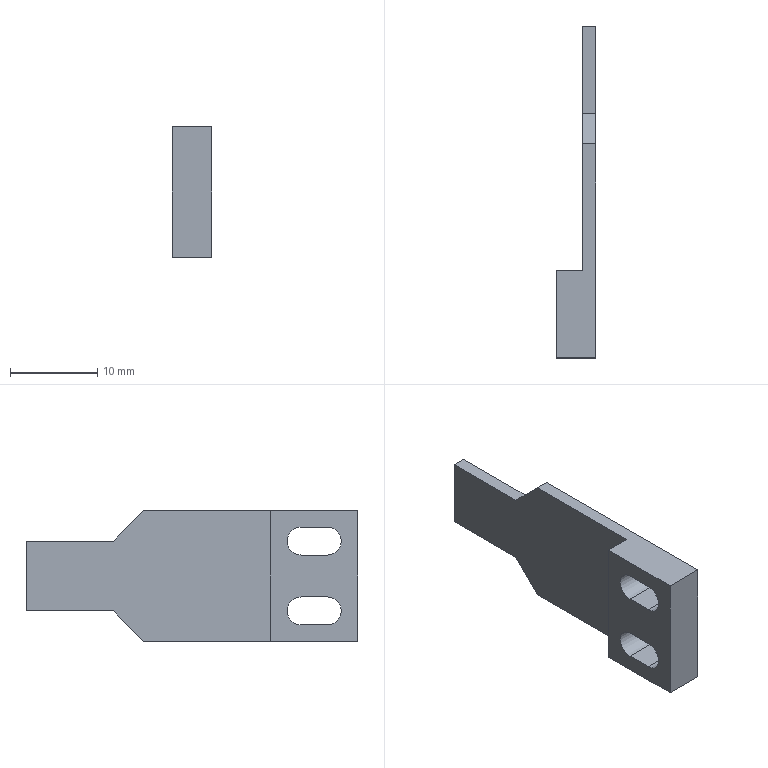Part | SolidWorks | features BaseBody 1 | 1 solid | 20 faces | box 4.5 x 38 x 15 mm | volume 1023 mm3 | plane 16 | cylinder 4 | commonest cylinder face diameters 3.2 x4
STEP:
#1=CARTESIAN_POINT('',(-50.496,1801.544,-58.1));
#2=VERTEX_POINT('',#1);
#3=CARTESIAN_POINT('',(-50.496,1798.544,-58.1));
#4=VERTEX_POINT('',#3);
#5=CARTESIAN_POINT('',(-50.496,1833.044,-58.1));
#6=DIRECTION('',(0.,-1.,0.));
#7=VECTOR('',#6,1000.);
#8=LINE('',#5,#7);
#9=EDGE_CURVE('',#2,#4,#8,.T.);
#10=ORIENTED_EDGE('',*,*,#9,.T.);
#11=CARTESIAN_POINT('',(-50.496,1798.544,-54.9));
#12=VERTEX_POINT('',#11);
#13=CARTESIAN_POINT('',(-50.496,1798.544,-56.5));
#14=DIRECTION('',(-1.,0.,0.));
#15=DIRECTION('',(0.,0.,-1.));
#16=AXIS2_PLACEMENT_3D('',#13,#14,#15);
#17=CIRCLE('',#16,1.6);
#18=EDGE_CURVE('',#4,#12,#17,.T.);
#19=ORIENTED_EDGE('',*,*,#18,.T.);
#20=CARTESIAN_POINT('',(-50.496,1801.544,-54.9));
#21=VERTEX_POINT('',#20);
#22=CARTESIAN_POINT('',(-50.496,1833.044,-54.9));
#23=DIRECTION('',(0.,1.,0.));
#24=VECTOR('',#23,1000.);
#25=LINE('',#22,#24);
#26=EDGE_CURVE('',#12,#21,#25,.T.);
#27=ORIENTED_EDGE('',*,*,#26,.T.);
#28=CARTESIAN_POINT('',(-50.496,1801.544,-56.5));
#29=DIRECTION('',(-1.,0.,0.));
#30=DIRECTION('',(0.,0.,-1.));
#31=AXIS2_PLACEMENT_3D('',#28,#29,#30);
#32=CIRCLE('',#31,1.6);
#33=EDGE_CURVE('',#21,#2,#32,.T.);
#34=ORIENTED_EDGE('',*,*,#33,.T.);
#35=EDGE_LOOP('',(#10,#19,#27,#34));
#36=FACE_BOUND('',#35,.T.);
#37=CARTESIAN_POINT('',(-50.496,1801.544,-66.1));
#38=VERTEX_POINT('',#37);
#39=CARTESIAN_POINT('',(-50.496,1798.544,-66.1));
#40=VERTEX_POINT('',#39);
#41=CARTESIAN_POINT('',(-50.496,1833.044,-66.1));
#42=DIRECTION('',(0.,-1.,0.));
#43=VECTOR('',#42,1000.);
#44=LINE('',#41,#43);
#45=EDGE_CURVE('',#38,#40,#44,.T.);
#46=ORIENTED_EDGE('',*,*,#45,.T.);
#47=CARTESIAN_POINT('',(-50.496,1798.544,-62.9));
#48=VERTEX_POINT('',#47);
#49=CARTESIAN_POINT('',(-50.496,1798.544,-64.5));
#50=DIRECTION('',(-1.,0.,0.));
#51=DIRECTION('',(0.,0.,-1.));
#52=AXIS2_PLACEMENT_3D('',#49,#50,#51);
#53=CIRCLE('',#52,1.6);
#54=EDGE_CURVE('',#40,#48,#53,.T.);
#55=ORIENTED_EDGE('',*,*,#54,.T.);
#56=CARTESIAN_POINT('',(-50.496,1801.544,-62.9));
#57=VERTEX_POINT('',#56);
#58=CARTESIAN_POINT('',(-50.496,1833.044,-62.9));
#59=DIRECTION('',(0.,1.,0.));
#60=VECTOR('',#59,1000.);
#61=LINE('',#58,#60);
#62=EDGE_CURVE('',#48,#57,#61,.T.);
#63=ORIENTED_EDGE('',*,*,#62,.T.);
#64=CARTESIAN_POINT('',(-50.496,1801.544,-64.5));
#65=DIRECTION('',(-1.,0.,0.));
#66=DIRECTION('',(0.,0.,-1.));
#67=AXIS2_PLACEMENT_3D('',#64,#65,#66);
#68=CIRCLE('',#67,1.6);
#69=EDGE_CURVE('',#57,#38,#68,.T.);
#70=ORIENTED_EDGE('',*,*,#69,.T.);
#71=EDGE_LOOP('',(#46,#55,#63,#70));
#72=FACE_BOUND('',#71,.T.);
#73=CARTESIAN_POINT('',(-50.496,1823.044,-64.5));
#74=VERTEX_POINT('',#73);
#75=CARTESIAN_POINT('',(-50.496,1833.044,-64.5));
#76=VERTEX_POINT('',#75);
#77=CARTESIAN_POINT('',(-50.496,1833.044,-64.5));
#78=DIRECTION('',(0.,1.,0.));
#79=VECTOR('',#78,1000.);
#80=LINE('',#77,#79);
#81=EDGE_CURVE('',#74,#76,#80,.T.);
#82=ORIENTED_EDGE('',*,*,#81,.T.);
#83=CARTESIAN_POINT('',(-50.496,1833.044,-56.5));
#84=VERTEX_POINT('',#83);
#85=CARTESIAN_POINT('',(-50.496,1833.044,-53.));
#86=DIRECTION('',(0.,0.,1.));
#87=VECTOR('',#86,1000.);
#88=LINE('',#85,#87);
#89=EDGE_CURVE('',#76,#84,#88,.T.);
#90=ORIENTED_EDGE('',*,*,#89,.T.);
#91=CARTESIAN_POINT('',(-50.496,1823.044,-56.5));
#92=VERTEX_POINT('',#91);
#93=CARTESIAN_POINT('',(-50.496,1833.044,-56.5));
#94=DIRECTION('',(0.,-1.,0.));
#95=VECTOR('',#94,1000.);
#96=LINE('',#93,#95);
#97=EDGE_CURVE('',#84,#92,#96,.T.);
#98=ORIENTED_EDGE('',*,*,#97,.T.);
#99=CARTESIAN_POINT('',(-50.496,1819.544,-53.));
#100=VERTEX_POINT('',#99);
#101=CARTESIAN_POINT('',(-50.496,1823.044,-56.5));
#102=DIRECTION('',(0.,-0.7071,0.7071));
#103=VECTOR('',#102,1000.);
#104=LINE('',#101,#103);
#105=EDGE_CURVE('',#92,#100,#104,.T.);
#106=ORIENTED_EDGE('',*,*,#105,.T.);
#107=CARTESIAN_POINT('',(-50.496,1795.044,-53.));
#108=VERTEX_POINT('',#107);
#109=CARTESIAN_POINT('',(-50.496,1833.044,-53.));
#110=DIRECTION('',(0.,-1.,0.));
#111=VECTOR('',#110,1000.);
#112=LINE('',#109,#111);
#113=EDGE_CURVE('',#100,#108,#112,.T.);
#114=ORIENTED_EDGE('',*,*,#113,.T.);
#115=CARTESIAN_POINT('',(-50.496,1795.044,-68.));
#116=VERTEX_POINT('',#115);
#117=CARTESIAN_POINT('',(-50.496,1795.044,-53.));
#118=DIRECTION('',(0.,0.,-1.));
#119=VECTOR('',#118,1000.);
#120=LINE('',#117,#119);
#121=EDGE_CURVE('',#108,#116,#120,.T.);
#122=ORIENTED_EDGE('',*,*,#121,.T.);
#123=CARTESIAN_POINT('',(-50.496,1819.544,-68.));
#124=VERTEX_POINT('',#123);
#125=CARTESIAN_POINT('',(-50.496,1833.044,-68.));
#126=DIRECTION('',(0.,1.,0.));
#127=VECTOR('',#126,1000.);
#128=LINE('',#125,#127);
#129=EDGE_CURVE('',#116,#124,#128,.T.);
#130=ORIENTED_EDGE('',*,*,#129,.T.);
#131=CARTESIAN_POINT('',(-50.496,1819.544,-68.));
#132=DIRECTION('',(0.,0.7071,0.7071));
#133=VECTOR('',#132,1000.);
#134=LINE('',#131,#133);
#135=EDGE_CURVE('',#124,#74,#134,.T.);
#136=ORIENTED_EDGE('',*,*,#135,.T.);
#137=EDGE_LOOP('',(#82,#90,#98,#106,#114,#122,#130,#136));
#138=FACE_OUTER_BOUND('',#137,.T.);
#139=CARTESIAN_POINT('',(-50.496,1833.044,-53.));
#140=DIRECTION('',(1.,0.,0.));
#141=DIRECTION('',(0.,0.,-1.));
#142=AXIS2_PLACEMENT_3D('',#139,#140,#141);
#143=PLANE('',#142);
#144=ADVANCED_FACE('',(#36,#72,#138),#143,.T.);
#145=CARTESIAN_POINT('',(-54.996,1798.544,-54.9));
#146=VERTEX_POINT('',#145);
#147=CARTESIAN_POINT('',(-54.996,1798.544,-58.1));
#148=VERTEX_POINT('',#147);
#149=CARTESIAN_POINT('',(-54.996,1798.544,-56.5));
#150=DIRECTION('',(1.,0.,0.));
#151=DIRECTION('',(0.,0.,-1.));
#152=AXIS2_PLACEMENT_3D('',#149,#150,#151);
#153=CIRCLE('',#152,1.6);
#154=EDGE_CURVE('',#146,#148,#153,.T.);
#155=ORIENTED_EDGE('',*,*,#154,.F.);
#156=CARTESIAN_POINT('',(-54.996,1798.544,-54.9));
#157=DIRECTION('',(-1.,0.,0.));
#158=VECTOR('',#157,1000.);
#159=LINE('',#156,#158);
#160=EDGE_CURVE('',#12,#146,#159,.T.);
#161=ORIENTED_EDGE('',*,*,#160,.F.);
#162=ORIENTED_EDGE('',*,*,#18,.F.);
#163=CARTESIAN_POINT('',(-54.996,1798.544,-58.1));
#164=DIRECTION('',(1.,0.,0.));
#165=VECTOR('',#164,1000.);
#166=LINE('',#163,#165);
#167=EDGE_CURVE('',#148,#4,#166,.T.);
#168=ORIENTED_EDGE('',*,*,#167,.F.);
#169=EDGE_LOOP('',(#155,#161,#162,#168));
#170=FACE_OUTER_BOUND('',#169,.T.);
#171=CARTESIAN_POINT('',(-54.996,1798.544,-56.5));
#172=DIRECTION('',(1.,0.,0.));
#173=DIRECTION('',(0.,0.,-1.));
#174=AXIS2_PLACEMENT_3D('',#171,#172,#173);
#175=CYLINDRICAL_SURFACE('',#174,1.6);
#176=ADVANCED_FACE('',(#170),#175,.F.);
#177=CARTESIAN_POINT('',(-54.996,1801.544,-58.1));
#178=VERTEX_POINT('',#177);
#179=CARTESIAN_POINT('',(-54.996,1798.544,-58.1));
#180=DIRECTION('',(0.,1.,0.));
#181=VECTOR('',#180,1000.);
#182=LINE('',#179,#181);
#183=EDGE_CURVE('',#148,#178,#182,.T.);
#184=ORIENTED_EDGE('',*,*,#183,.F.);
#185=ORIENTED_EDGE('',*,*,#167,.T.);
#186=ORIENTED_EDGE('',*,*,#9,.F.);
#187=CARTESIAN_POINT('',(-54.996,1801.544,-58.1));
#188=DIRECTION('',(1.,0.,0.));
#189=VECTOR('',#188,1000.);
#190=LINE('',#187,#189);
#191=EDGE_CURVE('',#178,#2,#190,.T.);
#192=ORIENTED_EDGE('',*,*,#191,.F.);
#193=EDGE_LOOP('',(#184,#185,#186,#192));
#194=FACE_OUTER_BOUND('',#193,.T.);
#195=CARTESIAN_POINT('',(-54.996,1798.544,-58.1));
#196=DIRECTION('',(0.,0.,-1.));
#197=DIRECTION('',(-1.,0.,0.));
#198=AXIS2_PLACEMENT_3D('',#195,#196,#197);
#199=PLANE('',#198);
#200=ADVANCED_FACE('',(#194),#199,.F.);
#201=CARTESIAN_POINT('',(-54.996,1801.544,-54.9));
#202=VERTEX_POINT('',#201);
#203=CARTESIAN_POINT('',(-54.996,1801.544,-56.5));
#204=DIRECTION('',(1.,0.,0.));
#205=DIRECTION('',(0.,0.,-1.));
#206=AXIS2_PLACEMENT_3D('',#203,#204,#205);
#207=CIRCLE('',#206,1.6);
#208=EDGE_CURVE('',#178,#202,#207,.T.);
#209=ORIENTED_EDGE('',*,*,#208,.F.);
#210=ORIENTED_EDGE('',*,*,#191,.T.);
#211=ORIENTED_EDGE('',*,*,#33,.F.);
#212=CARTESIAN_POINT('',(-54.996,1801.544,-54.9));
#213=DIRECTION('',(1.,0.,0.));
#214=VECTOR('',#213,1000.);
#215=LINE('',#212,#214);
#216=EDGE_CURVE('',#202,#21,#215,.T.);
#217=ORIENTED_EDGE('',*,*,#216,.F.);
#218=EDGE_LOOP('',(#209,#210,#211,#217));
#219=FACE_OUTER_BOUND('',#218,.T.);
#220=CARTESIAN_POINT('',(-54.996,1801.544,-56.5));
#221=DIRECTION('',(1.,0.,0.));
#222=DIRECTION('',(0.,0.,-1.));
#223=AXIS2_PLACEMENT_3D('',#220,#221,#222);
#224=CYLINDRICAL_SURFACE('',#223,1.6);
#225=ADVANCED_FACE('',(#219),#224,.F.);
#226=CARTESIAN_POINT('',(-54.996,1798.544,-54.9));
#227=DIRECTION('',(0.,-1.,0.));
#228=VECTOR('',#227,1000.);
#229=LINE('',#226,#228);
#230=EDGE_CURVE('',#202,#146,#229,.T.);
#231=ORIENTED_EDGE('',*,*,#230,.F.);
#232=ORIENTED_EDGE('',*,*,#216,.T.);
#233=ORIENTED_EDGE('',*,*,#26,.F.);
#234=ORIENTED_EDGE('',*,*,#160,.T.);
#235=EDGE_LOOP('',(#231,#232,#233,#234));
#236=FACE_OUTER_BOUND('',#235,.T.);
#237=CARTESIAN_POINT('',(-54.996,1798.544,-54.9));
#238=DIRECTION('',(0.,0.,1.));
#239=DIRECTION('',(1.,0.,0.));
#240=AXIS2_PLACEMENT_3D('',#237,#238,#239);
#241=PLANE('',#240);
#242=ADVANCED_FACE('',(#236),#241,.F.);
#243=CARTESIAN_POINT('',(-54.996,1798.544,-62.9));
#244=VERTEX_POINT('',#243);
#245=CARTESIAN_POINT('',(-54.996,1798.544,-66.1));
#246=VERTEX_POINT('',#245);
#247=CARTESIAN_POINT('',(-54.996,1798.544,-64.5));
#248=DIRECTION('',(1.,0.,0.));
#249=DIRECTION('',(0.,0.,-1.));
#250=AXIS2_PLACEMENT_3D('',#247,#248,#249);
#251=CIRCLE('',#250,1.6);
#252=EDGE_CURVE('',#244,#246,#251,.T.);
#253=ORIENTED_EDGE('',*,*,#252,.F.);
#254=CARTESIAN_POINT('',(-54.996,1798.544,-62.9));
#255=DIRECTION('',(-1.,0.,0.));
#256=VECTOR('',#255,1000.);
#257=LINE('',#254,#256);
#258=EDGE_CURVE('',#48,#244,#257,.T.);
#259=ORIENTED_EDGE('',*,*,#258,.F.);
#260=ORIENTED_EDGE('',*,*,#54,.F.);
#261=CARTESIAN_POINT('',(-54.996,1798.544,-66.1));
#262=DIRECTION('',(1.,0.,0.));
#263=VECTOR('',#262,1000.);
#264=LINE('',#261,#263);
#265=EDGE_CURVE('',#246,#40,#264,.T.);
#266=ORIENTED_EDGE('',*,*,#265,.F.);
#267=EDGE_LOOP('',(#253,#259,#260,#266));
#268=FACE_OUTER_BOUND('',#267,.T.);
#269=CARTESIAN_POINT('',(-54.996,1798.544,-64.5));
#270=DIRECTION('',(1.,0.,0.));
#271=DIRECTION('',(0.,0.,-1.));
#272=AXIS2_PLACEMENT_3D('',#269,#270,#271);
#273=CYLINDRICAL_SURFACE('',#272,1.6);
#274=ADVANCED_FACE('',(#268),#273,.F.);
#275=CARTESIAN_POINT('',(-54.996,1801.544,-66.1));
#276=VERTEX_POINT('',#275);
#277=CARTESIAN_POINT('',(-54.996,1798.544,-66.1));
#278=DIRECTION('',(0.,1.,0.));
#279=VECTOR('',#278,1000.);
#280=LINE('',#277,#279);
#281=EDGE_CURVE('',#246,#276,#280,.T.);
#282=ORIENTED_EDGE('',*,*,#281,.F.);
#283=ORIENTED_EDGE('',*,*,#265,.T.);
#284=ORIENTED_EDGE('',*,*,#45,.F.);
#285=CARTESIAN_POINT('',(-54.996,1801.544,-66.1));
#286=DIRECTION('',(1.,0.,0.));
#287=VECTOR('',#286,1000.);
#288=LINE('',#285,#287);
#289=EDGE_CURVE('',#276,#38,#288,.T.);
#290=ORIENTED_EDGE('',*,*,#289,.F.);
#291=EDGE_LOOP('',(#282,#283,#284,#290));
#292=FACE_OUTER_BOUND('',#291,.T.);
#293=CARTESIAN_POINT('',(-54.996,1798.544,-66.1));
#294=DIRECTION('',(0.,0.,-1.));
#295=DIRECTION('',(-1.,0.,0.));
#296=AXIS2_PLACEMENT_3D('',#293,#294,#295);
#297=PLANE('',#296);
#298=ADVANCED_FACE('',(#292),#297,.F.);
#299=CARTESIAN_POINT('',(-54.996,1801.544,-62.9));
#300=VERTEX_POINT('',#299);
#301=CARTESIAN_POINT('',(-54.996,1801.544,-64.5));
#302=DIRECTION('',(1.,0.,0.));
#303=DIRECTION('',(0.,0.,-1.));
#304=AXIS2_PLACEMENT_3D('',#301,#302,#303);
#305=CIRCLE('',#304,1.6);
#306=EDGE_CURVE('',#276,#300,#305,.T.);
#307=ORIENTED_EDGE('',*,*,#306,.F.);
#308=ORIENTED_EDGE('',*,*,#289,.T.);
#309=ORIENTED_EDGE('',*,*,#69,.F.);
#310=CARTESIAN_POINT('',(-54.996,1801.544,-62.9));
#311=DIRECTION('',(1.,0.,0.));
#312=VECTOR('',#311,1000.);
#313=LINE('',#310,#312);
#314=EDGE_CURVE('',#300,#57,#313,.T.);
#315=ORIENTED_EDGE('',*,*,#314,.F.);
#316=EDGE_LOOP('',(#307,#308,#309,#315));
#317=FACE_OUTER_BOUND('',#316,.T.);
#318=CARTESIAN_POINT('',(-54.996,1801.544,-64.5));
#319=DIRECTION('',(1.,0.,0.));
#320=DIRECTION('',(0.,0.,-1.));
#321=AXIS2_PLACEMENT_3D('',#318,#319,#320);
#322=CYLINDRICAL_SURFACE('',#321,1.6);
#323=ADVANCED_FACE('',(#317),#322,.F.);
#324=CARTESIAN_POINT('',(-54.996,1798.544,-62.9));
#325=DIRECTION('',(0.,-1.,0.));
#326=VECTOR('',#325,1000.);
#327=LINE('',#324,#326);
#328=EDGE_CURVE('',#300,#244,#327,.T.);
#329=ORIENTED_EDGE('',*,*,#328,.F.);
#330=ORIENTED_EDGE('',*,*,#314,.T.);
#331=ORIENTED_EDGE('',*,*,#62,.F.);
#332=ORIENTED_EDGE('',*,*,#258,.T.);
#333=EDGE_LOOP('',(#329,#330,#331,#332));
#334=FACE_OUTER_BOUND('',#333,.T.);
#335=CARTESIAN_POINT('',(-54.996,1798.544,-62.9));
#336=DIRECTION('',(0.,0.,1.));
#337=DIRECTION('',(1.,0.,0.));
#338=AXIS2_PLACEMENT_3D('',#335,#336,#337);
#339=PLANE('',#338);
#340=ADVANCED_FACE('',(#334),#339,.F.);
#341=CARTESIAN_POINT('',(-51.996,1833.044,-64.5));
#342=VERTEX_POINT('',#341);
#343=CARTESIAN_POINT('',(-51.996,1833.044,-64.5));
#344=DIRECTION('',(-1.,0.,0.));
#345=VECTOR('',#344,1000.);
#346=LINE('',#343,#345);
#347=EDGE_CURVE('',#76,#342,#346,.T.);
#348=ORIENTED_EDGE('',*,*,#347,.T.);
#349=CARTESIAN_POINT('',(-51.996,1833.044,-56.5));
#350=VERTEX_POINT('',#349);
#351=CARTESIAN_POINT('',(-51.996,1833.044,-53.));
#352=DIRECTION('',(0.,0.,1.));
#353=VECTOR('',#352,1000.);
#354=LINE('',#351,#353);
#355=EDGE_CURVE('',#342,#350,#354,.T.);
#356=ORIENTED_EDGE('',*,*,#355,.T.);
#357=CARTESIAN_POINT('',(-51.996,1833.044,-56.5));
#358=DIRECTION('',(1.,0.,0.));
#359=VECTOR('',#358,1000.);
#360=LINE('',#357,#359);
#361=EDGE_CURVE('',#350,#84,#360,.T.);
#362=ORIENTED_EDGE('',*,*,#361,.T.);
#363=ORIENTED_EDGE('',*,*,#89,.F.);
#364=EDGE_LOOP('',(#348,#356,#362,#363));
#365=FACE_OUTER_BOUND('',#364,.T.);
#366=CARTESIAN_POINT('',(-51.996,1833.044,-53.));
#367=DIRECTION('',(0.,1.,0.));
#368=DIRECTION('',(0.,0.,1.));
#369=AXIS2_PLACEMENT_3D('',#366,#367,#368);
#370=PLANE('',#369);
#371=ADVANCED_FACE('',(#365),#370,.T.);
#372=ORIENTED_EDGE('',*,*,#81,.F.);
#373=CARTESIAN_POINT('',(-51.996,1823.044,-64.5));
#374=VERTEX_POINT('',#373);
#375=CARTESIAN_POINT('',(-54.996,1823.044,-64.5));
#376=DIRECTION('',(1.,0.,0.));
#377=VECTOR('',#376,1000.);
#378=LINE('',#375,#377);
#379=EDGE_CURVE('',#374,#74,#378,.T.);
#380=ORIENTED_EDGE('',*,*,#379,.F.);
#381=CARTESIAN_POINT('',(-51.996,1823.044,-64.5));
#382=DIRECTION('',(0.,-1.,0.));
#383=VECTOR('',#382,1000.);
#384=LINE('',#381,#383);
#385=EDGE_CURVE('',#342,#374,#384,.T.);
#386=ORIENTED_EDGE('',*,*,#385,.F.);
#387=ORIENTED_EDGE('',*,*,#347,.F.);
#388=EDGE_LOOP('',(#372,#380,#386,#387));
#389=FACE_OUTER_BOUND('',#388,.T.);
#390=CARTESIAN_POINT('',(-54.996,1823.044,-64.5));
#391=DIRECTION('',(0.,0.,1.));
#392=DIRECTION('',(1.,0.,0.));
#393=AXIS2_PLACEMENT_3D('',#390,#391,#392);
#394=PLANE('',#393);
#395=ADVANCED_FACE('',(#389),#394,.F.);
#396=ORIENTED_EDGE('',*,*,#135,.F.);
#397=CARTESIAN_POINT('',(-51.996,1819.544,-68.));
#398=VERTEX_POINT('',#397);
#399=CARTESIAN_POINT('',(-54.996,1819.544,-68.));
#400=DIRECTION('',(1.,0.,0.));
#401=VECTOR('',#400,1000.);
#402=LINE('',#399,#401);
#403=EDGE_CURVE('',#398,#124,#402,.T.);
#404=ORIENTED_EDGE('',*,*,#403,.F.);
#405=CARTESIAN_POINT('',(-51.996,1819.544,-68.));
#406=DIRECTION('',(0.,-0.7071,-0.7071));
#407=VECTOR('',#406,1000.);
#408=LINE('',#405,#407);
#409=EDGE_CURVE('',#374,#398,#408,.T.);
#410=ORIENTED_EDGE('',*,*,#409,.F.);
#411=ORIENTED_EDGE('',*,*,#379,.T.);
#412=EDGE_LOOP('',(#396,#404,#410,#411));
#413=FACE_OUTER_BOUND('',#412,.T.);
#414=CARTESIAN_POINT('',(-54.996,1819.544,-68.));
#415=DIRECTION('',(0.,-0.7071,0.7071));
#416=DIRECTION('',(0.,-0.7071,-0.7071));
#417=AXIS2_PLACEMENT_3D('',#414,#415,#416);
#418=PLANE('',#417);
#419=ADVANCED_FACE('',(#413),#418,.F.);
#420=CARTESIAN_POINT('',(-51.996,1805.044,-68.));
#421=VERTEX_POINT('',#420);
#422=CARTESIAN_POINT('',(-51.996,1833.044,-68.));
#423=DIRECTION('',(0.,1.,0.));
#424=VECTOR('',#423,1000.);
#425=LINE('',#422,#424);
#426=EDGE_CURVE('',#421,#398,#425,.T.);
#427=ORIENTED_EDGE('',*,*,#426,.T.);
#428=ORIENTED_EDGE('',*,*,#403,.T.);
#429=ORIENTED_EDGE('',*,*,#129,.F.);
#430=CARTESIAN_POINT('',(-54.996,1795.044,-68.));
#431=VERTEX_POINT('',#430);
#432=CARTESIAN_POINT('',(-50.496,1795.044,-68.));
#433=DIRECTION('',(-1.,0.,0.));
#434=VECTOR('',#433,1000.);
#435=LINE('',#432,#434);
#436=EDGE_CURVE('',#116,#431,#435,.T.);
#437=ORIENTED_EDGE('',*,*,#436,.T.);
#438=CARTESIAN_POINT('',(-54.996,1805.044,-68.));
#439=VERTEX_POINT('',#438);
#440=CARTESIAN_POINT('',(-54.996,1833.044,-68.));
#441=DIRECTION('',(0.,1.,0.));
#442=VECTOR('',#441,1000.);
#443=LINE('',#440,#442);
#444=EDGE_CURVE('',#431,#439,#443,.T.);
#445=ORIENTED_EDGE('',*,*,#444,.T.);
#446=CARTESIAN_POINT('',(-50.496,1805.044,-68.));
#447=DIRECTION('',(1.,0.,0.));
#448=VECTOR('',#447,1000.);
#449=LINE('',#446,#448);
#450=EDGE_CURVE('',#439,#421,#449,.T.);
#451=ORIENTED_EDGE('',*,*,#450,.T.);
#452=EDGE_LOOP('',(#427,#428,#429,#437,#445,#451));
#453=FACE_OUTER_BOUND('',#452,.T.);
#454=CARTESIAN_POINT('',(-50.496,1833.044,-68.));
#455=DIRECTION('',(0.,0.,-1.));
#456=DIRECTION('',(-1.,0.,0.));
#457=AXIS2_PLACEMENT_3D('',#454,#455,#456);
#458=PLANE('',#457);
#459=ADVANCED_FACE('',(#453),#458,.T.);
#460=CARTESIAN_POINT('',(-54.996,1795.044,-53.));
#461=VERTEX_POINT('',#460);
#462=CARTESIAN_POINT('',(-54.996,1795.044,-53.));
#463=DIRECTION('',(0.,0.,-1.));
#464=VECTOR('',#463,1000.);
#465=LINE('',#462,#464);
#466=EDGE_CURVE('',#461,#431,#465,.T.);
#467=ORIENTED_EDGE('',*,*,#466,.T.);
#468=ORIENTED_EDGE('',*,*,#436,.F.);
#469=ORIENTED_EDGE('',*,*,#121,.F.);
#470=CARTESIAN_POINT('',(-50.496,1795.044,-53.));
#471=DIRECTION('',(-1.,0.,0.));
#472=VECTOR('',#471,1000.);
#473=LINE('',#470,#472);
#474=EDGE_CURVE('',#108,#461,#473,.T.);
#475=ORIENTED_EDGE('',*,*,#474,.T.);
#476=EDGE_LOOP('',(#467,#468,#469,#475));
#477=FACE_OUTER_BOUND('',#476,.T.);
#478=CARTESIAN_POINT('',(-50.496,1795.044,-53.));
#479=DIRECTION('',(0.,-1.,0.));
#480=DIRECTION('',(0.,0.,-1.));
#481=AXIS2_PLACEMENT_3D('',#478,#479,#480);
#482=PLANE('',#481);
#483=ADVANCED_FACE('',(#477),#482,.T.);
#484=CARTESIAN_POINT('',(-54.996,1805.044,-53.));
#485=VERTEX_POINT('',#484);
#486=CARTESIAN_POINT('',(-51.996,1805.044,-53.));
#487=VERTEX_POINT('',#486);
#488=CARTESIAN_POINT('',(-50.496,1805.044,-53.));
#489=DIRECTION('',(1.,0.,0.));
#490=VECTOR('',#489,1000.);
#491=LINE('',#488,#490);
#492=EDGE_CURVE('',#485,#487,#491,.T.);
#493=ORIENTED_EDGE('',*,*,#492,.F.);
#494=CARTESIAN_POINT('',(-54.996,1833.044,-53.));
#495=DIRECTION('',(0.,1.,0.));
#496=VECTOR('',#495,1000.);
#497=LINE('',#494,#496);
#498=EDGE_CURVE('',#461,#485,#497,.T.);
#499=ORIENTED_EDGE('',*,*,#498,.F.);
#500=ORIENTED_EDGE('',*,*,#474,.F.);
#501=ORIENTED_EDGE('',*,*,#113,.F.);
#502=CARTESIAN_POINT('',(-51.996,1819.544,-53.));
#503=VERTEX_POINT('',#502);
#504=CARTESIAN_POINT('',(-50.496,1819.544,-53.));
#505=DIRECTION('',(1.,0.,0.));
#506=VECTOR('',#505,1000.);
#507=LINE('',#504,#506);
#508=EDGE_CURVE('',#503,#100,#507,.T.);
#509=ORIENTED_EDGE('',*,*,#508,.F.);
#510=CARTESIAN_POINT('',(-51.996,1833.044,-53.));
#511=DIRECTION('',(0.,1.,0.));
#512=VECTOR('',#511,1000.);
#513=LINE('',#510,#512);
#514=EDGE_CURVE('',#487,#503,#513,.T.);
#515=ORIENTED_EDGE('',*,*,#514,.F.);
#516=EDGE_LOOP('',(#493,#499,#500,#501,#509,#515));
#517=FACE_OUTER_BOUND('',#516,.T.);
#518=CARTESIAN_POINT('',(-50.496,1833.044,-53.));
#519=DIRECTION('',(0.,0.,-1.));
#520=DIRECTION('',(-1.,0.,0.));
#521=AXIS2_PLACEMENT_3D('',#518,#519,#520);
#522=PLANE('',#521);
#523=ADVANCED_FACE('',(#517),#522,.F.);
#524=CARTESIAN_POINT('',(-51.996,1823.044,-56.5));
#525=VERTEX_POINT('',#524);
#526=CARTESIAN_POINT('',(-51.996,1819.544,-53.));
#527=DIRECTION('',(0.,-0.7071,0.7071));
#528=VECTOR('',#527,1000.);
#529=LINE('',#526,#528);
#530=EDGE_CURVE('',#525,#503,#529,.T.);
#531=ORIENTED_EDGE('',*,*,#530,.T.);
#532=ORIENTED_EDGE('',*,*,#508,.T.);
#533=ORIENTED_EDGE('',*,*,#105,.F.);
#534=CARTESIAN_POINT('',(-54.996,1823.044,-56.5));
#535=DIRECTION('',(-1.,0.,0.));
#536=VECTOR('',#535,1000.);
#537=LINE('',#534,#536);
#538=EDGE_CURVE('',#92,#525,#537,.T.);
#539=ORIENTED_EDGE('',*,*,#538,.T.);
#540=EDGE_LOOP('',(#531,#532,#533,#539));
#541=FACE_OUTER_BOUND('',#540,.T.);
#542=CARTESIAN_POINT('',(-54.996,1819.544,-53.));
#543=DIRECTION('',(0.,0.7071,0.7071));
#544=DIRECTION('',(0.,-0.7071,0.7071));
#545=AXIS2_PLACEMENT_3D('',#542,#543,#544);
#546=PLANE('',#545);
#547=ADVANCED_FACE('',(#541),#546,.T.);
#548=CARTESIAN_POINT('',(-51.996,1823.044,-56.5));
#549=DIRECTION('',(0.,-1.,0.));
#550=VECTOR('',#549,1000.);
#551=LINE('',#548,#550);
#552=EDGE_CURVE('',#350,#525,#551,.T.);
#553=ORIENTED_EDGE('',*,*,#552,.T.);
#554=ORIENTED_EDGE('',*,*,#538,.F.);
#555=ORIENTED_EDGE('',*,*,#97,.F.);
#556=ORIENTED_EDGE('',*,*,#361,.F.);
#557=EDGE_LOOP('',(#553,#554,#555,#556));
#558=FACE_OUTER_BOUND('',#557,.T.);
#559=CARTESIAN_POINT('',(-54.996,1823.044,-56.5));
#560=DIRECTION('',(0.,0.,1.));
#561=DIRECTION('',(1.,0.,0.));
#562=AXIS2_PLACEMENT_3D('',#559,#560,#561);
#563=PLANE('',#562);
#564=ADVANCED_FACE('',(#558),#563,.T.);
#565=ORIENTED_EDGE('',*,*,#230,.T.);
#566=ORIENTED_EDGE('',*,*,#154,.T.);
#567=ORIENTED_EDGE('',*,*,#183,.T.);
#568=ORIENTED_EDGE('',*,*,#208,.T.);
#569=EDGE_LOOP('',(#565,#566,#567,#568));
#570=FACE_BOUND('',#569,.T.);
#571=ORIENTED_EDGE('',*,*,#328,.T.);
#572=ORIENTED_EDGE('',*,*,#252,.T.);
#573=ORIENTED_EDGE('',*,*,#281,.T.);
#574=ORIENTED_EDGE('',*,*,#306,.T.);
#575=EDGE_LOOP('',(#571,#572,#573,#574));
#576=FACE_BOUND('',#575,.T.);
#577=CARTESIAN_POINT('',(-54.996,1805.044,-53.));
#578=DIRECTION('',(0.,0.,-1.));
#579=VECTOR('',#578,1000.);
#580=LINE('',#577,#579);
#581=EDGE_CURVE('',#485,#439,#580,.T.);
#582=ORIENTED_EDGE('',*,*,#581,.T.);
#583=ORIENTED_EDGE('',*,*,#444,.F.);
#584=ORIENTED_EDGE('',*,*,#466,.F.);
#585=ORIENTED_EDGE('',*,*,#498,.T.);
#586=EDGE_LOOP('',(#582,#583,#584,#585));
#587=FACE_OUTER_BOUND('',#586,.T.);
#588=CARTESIAN_POINT('',(-54.996,1795.044,-53.));
#589=DIRECTION('',(-1.,0.,0.));
#590=DIRECTION('',(0.,0.,1.));
#591=AXIS2_PLACEMENT_3D('',#588,#589,#590);
#592=PLANE('',#591);
#593=ADVANCED_FACE('',(#570,#576,#587),#592,.T.);
#594=ORIENTED_EDGE('',*,*,#514,.T.);
#595=ORIENTED_EDGE('',*,*,#530,.F.);
#596=ORIENTED_EDGE('',*,*,#552,.F.);
#597=ORIENTED_EDGE('',*,*,#355,.F.);
#598=ORIENTED_EDGE('',*,*,#385,.T.);
#599=ORIENTED_EDGE('',*,*,#409,.T.);
#600=ORIENTED_EDGE('',*,*,#426,.F.);
#601=CARTESIAN_POINT('',(-51.996,1805.044,-53.));
#602=DIRECTION('',(0.,0.,1.));
#603=VECTOR('',#602,1000.);
#604=LINE('',#601,#603);
#605=EDGE_CURVE('',#421,#487,#604,.T.);
#606=ORIENTED_EDGE('',*,*,#605,.T.);
#607=EDGE_LOOP('',(#594,#595,#596,#597,#598,#599,#600,#606));
#608=FACE_OUTER_BOUND('',#607,.T.);
#609=CARTESIAN_POINT('',(-51.996,1805.044,-53.));
#610=DIRECTION('',(-1.,0.,0.));
#611=DIRECTION('',(0.,0.,1.));
#612=AXIS2_PLACEMENT_3D('',#609,#610,#611);
#613=PLANE('',#612);
#614=ADVANCED_FACE('',(#608),#613,.T.);
#615=ORIENTED_EDGE('',*,*,#605,.F.);
#616=ORIENTED_EDGE('',*,*,#450,.F.);
#617=ORIENTED_EDGE('',*,*,#581,.F.);
#618=ORIENTED_EDGE('',*,*,#492,.T.);
#619=EDGE_LOOP('',(#615,#616,#617,#618));
#620=FACE_OUTER_BOUND('',#619,.T.);
#621=CARTESIAN_POINT('',(-54.996,1805.044,-53.));
#622=DIRECTION('',(0.,1.,0.));
#623=DIRECTION('',(0.,0.,1.));
#624=AXIS2_PLACEMENT_3D('',#621,#622,#623);
#625=PLANE('',#624);
#626=ADVANCED_FACE('',(#620),#625,.T.);
#627=CLOSED_SHELL('',(#144,#176,#200,#225,#242,#274,#298,#323,#340,#371,#395,#419,#459,#483,#523,#547,#564,#593,#614,#626));
#628=MANIFOLD_SOLID_BREP('',#627);
#629=CARTESIAN_POINT('',(0.,0.,0.));
#630=DIRECTION('',(0.,0.,1.));
#631=DIRECTION('',(1.,0.,0.));
#632=AXIS2_PLACEMENT_3D('',#629,#630,#631);
#633=(LENGTH_UNIT()NAMED_UNIT(*)SI_UNIT(.MILLI.,.METRE.));
#634=UNCERTAINTY_MEASURE_WITH_UNIT(LENGTH_MEASURE(0.00001),#633,'','');
#635=(NAMED_UNIT(*)PLANE_ANGLE_UNIT()SI_UNIT($,.RADIAN.));
#636=(NAMED_UNIT(*)SI_UNIT($,.STERADIAN.)SOLID_ANGLE_UNIT());
#637=(GEOMETRIC_REPRESENTATION_CONTEXT(3)GLOBAL_UNCERTAINTY_ASSIGNED_CONTEXT((#634))GLOBAL_UNIT_ASSIGNED_CONTEXT((#633,#635,#636))REPRESENTATION_CONTEXT('',''));
#638=ADVANCED_BREP_SHAPE_REPRESENTATION('',(#628,#632),#637);